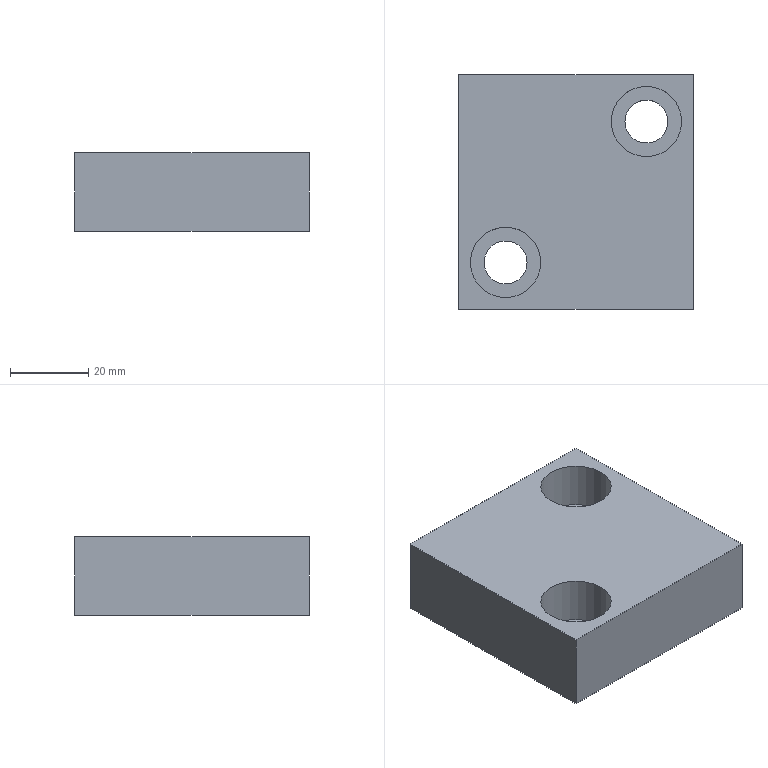Part | NX | features solid 2 | 1 solid | 12 faces | box 60 x 60 x 20 mm | volume 64372 mm3 | plane 8 | cylinder 4 | commonest cylinder face diameters 11 x2 18 x2
STEP:
#1=CARTESIAN_POINT('',(12.5,568.,142.));
#2=VERTEX_POINT('',#1);
#3=CARTESIAN_POINT('',(18.,568.,142.));
#4=DIRECTION('',(0.,0.,-1.));
#5=DIRECTION('',(-1.,0.,0.));
#6=AXIS2_PLACEMENT_3D('',#3,#4,#5);
#7=CIRCLE('',#6,5.5);
#8=EDGE_CURVE('',#2,#2,#7,.T.);
#9=ORIENTED_EDGE('',*,*,#8,.F.);
#10=EDGE_LOOP('',(#9));
#11=FACE_BOUND('',#10,.T.);
#12=CARTESIAN_POINT('',(-23.5,532.,142.));
#13=VERTEX_POINT('',#12);
#14=CARTESIAN_POINT('',(-18.,532.,142.));
#15=DIRECTION('',(0.,0.,-1.));
#16=DIRECTION('',(-1.,0.,0.));
#17=AXIS2_PLACEMENT_3D('',#14,#15,#16);
#18=CIRCLE('',#17,5.5);
#19=EDGE_CURVE('',#13,#13,#18,.T.);
#20=ORIENTED_EDGE('',*,*,#19,.F.);
#21=EDGE_LOOP('',(#20));
#22=FACE_BOUND('',#21,.T.);
#23=CARTESIAN_POINT('',(-30.,520.,142.));
#24=VERTEX_POINT('',#23);
#25=CARTESIAN_POINT('',(30.,520.,142.));
#26=VERTEX_POINT('',#25);
#27=CARTESIAN_POINT('',(-37.5,520.,142.));
#28=DIRECTION('',(-1.,0.,0.));
#29=VECTOR('',#28,1000.);
#30=LINE('',#27,#29);
#31=EDGE_CURVE('',#24,#26,#30,.F.);
#32=ORIENTED_EDGE('',*,*,#31,.F.);
#33=CARTESIAN_POINT('',(-30.,580.,142.));
#34=VERTEX_POINT('',#33);
#35=CARTESIAN_POINT('',(-30.,600.,142.));
#36=DIRECTION('',(0.,1.,0.));
#37=VECTOR('',#36,1000.);
#38=LINE('',#35,#37);
#39=EDGE_CURVE('',#34,#24,#38,.F.);
#40=ORIENTED_EDGE('',*,*,#39,.F.);
#41=CARTESIAN_POINT('',(30.,580.,142.));
#42=VERTEX_POINT('',#41);
#43=CARTESIAN_POINT('',(-37.5,580.,142.));
#44=DIRECTION('',(1.,0.,0.));
#45=VECTOR('',#44,1000.);
#46=LINE('',#43,#45);
#47=EDGE_CURVE('',#34,#42,#46,.T.);
#48=ORIENTED_EDGE('',*,*,#47,.T.);
#49=CARTESIAN_POINT('',(30.,600.,142.));
#50=DIRECTION('',(0.,-1.,0.));
#51=VECTOR('',#50,1000.);
#52=LINE('',#49,#51);
#53=EDGE_CURVE('',#42,#26,#52,.T.);
#54=ORIENTED_EDGE('',*,*,#53,.T.);
#55=EDGE_LOOP('',(#32,#40,#48,#54));
#56=FACE_BOUND('',#55,.T.);
#57=CARTESIAN_POINT('',(-37.5,600.,142.));
#58=DIRECTION('',(0.,0.,-1.));
#59=DIRECTION('',(-1.,0.,0.));
#60=AXIS2_PLACEMENT_3D('',#57,#58,#59);
#61=PLANE('',#60);
#62=ADVANCED_FACE('',(#11,#22,#56),#61,.T.);
#63=CARTESIAN_POINT('',(30.,580.,162.));
#64=VERTEX_POINT('',#63);
#65=CARTESIAN_POINT('',(30.,580.,142.));
#66=DIRECTION('',(0.,0.,1.));
#67=VECTOR('',#66,1000.);
#68=LINE('',#65,#67);
#69=EDGE_CURVE('',#42,#64,#68,.T.);
#70=ORIENTED_EDGE('',*,*,#69,.F.);
#71=ORIENTED_EDGE('',*,*,#47,.F.);
#72=CARTESIAN_POINT('',(-30.,580.,162.));
#73=VERTEX_POINT('',#72);
#74=CARTESIAN_POINT('',(-30.,580.,142.));
#75=DIRECTION('',(0.,0.,-1.));
#76=VECTOR('',#75,1000.);
#77=LINE('',#74,#76);
#78=EDGE_CURVE('',#34,#73,#77,.F.);
#79=ORIENTED_EDGE('',*,*,#78,.T.);
#80=CARTESIAN_POINT('',(-37.5,580.,162.));
#81=DIRECTION('',(1.,0.,0.));
#82=VECTOR('',#81,1000.);
#83=LINE('',#80,#82);
#84=EDGE_CURVE('',#73,#64,#83,.T.);
#85=ORIENTED_EDGE('',*,*,#84,.T.);
#86=EDGE_LOOP('',(#70,#71,#79,#85));
#87=FACE_BOUND('',#86,.T.);
#88=CARTESIAN_POINT('',(-37.5,580.,142.));
#89=DIRECTION('',(0.,1.,0.));
#90=DIRECTION('',(1.,0.,0.));
#91=AXIS2_PLACEMENT_3D('',#88,#89,#90);
#92=PLANE('',#91);
#93=ADVANCED_FACE('',(#87),#92,.T.);
#94=ORIENTED_EDGE('',*,*,#78,.F.);
#95=ORIENTED_EDGE('',*,*,#39,.T.);
#96=CARTESIAN_POINT('',(-30.,520.,162.));
#97=VERTEX_POINT('',#96);
#98=CARTESIAN_POINT('',(-30.,520.,142.));
#99=DIRECTION('',(0.,0.,1.));
#100=VECTOR('',#99,1000.);
#101=LINE('',#98,#100);
#102=EDGE_CURVE('',#24,#97,#101,.T.);
#103=ORIENTED_EDGE('',*,*,#102,.T.);
#104=CARTESIAN_POINT('',(-30.,600.,162.));
#105=DIRECTION('',(0.,1.,0.));
#106=VECTOR('',#105,1000.);
#107=LINE('',#104,#106);
#108=EDGE_CURVE('',#73,#97,#107,.F.);
#109=ORIENTED_EDGE('',*,*,#108,.F.);
#110=EDGE_LOOP('',(#94,#95,#103,#109));
#111=FACE_BOUND('',#110,.T.);
#112=CARTESIAN_POINT('',(-30.,600.,142.));
#113=DIRECTION('',(1.,0.,0.));
#114=DIRECTION('',(0.,-1.,0.));
#115=AXIS2_PLACEMENT_3D('',#112,#113,#114);
#116=PLANE('',#115);
#117=ADVANCED_FACE('',(#111),#116,.F.);
#118=ORIENTED_EDGE('',*,*,#102,.F.);
#119=ORIENTED_EDGE('',*,*,#31,.T.);
#120=CARTESIAN_POINT('',(30.,520.,162.));
#121=VERTEX_POINT('',#120);
#122=CARTESIAN_POINT('',(30.,520.,142.));
#123=DIRECTION('',(0.,0.,-1.));
#124=VECTOR('',#123,1000.);
#125=LINE('',#122,#124);
#126=EDGE_CURVE('',#26,#121,#125,.F.);
#127=ORIENTED_EDGE('',*,*,#126,.T.);
#128=CARTESIAN_POINT('',(-37.5,520.,162.));
#129=DIRECTION('',(-1.,0.,0.));
#130=VECTOR('',#129,1000.);
#131=LINE('',#128,#130);
#132=EDGE_CURVE('',#97,#121,#131,.F.);
#133=ORIENTED_EDGE('',*,*,#132,.F.);
#134=EDGE_LOOP('',(#118,#119,#127,#133));
#135=FACE_BOUND('',#134,.T.);
#136=CARTESIAN_POINT('',(-37.5,520.,142.));
#137=DIRECTION('',(0.,1.,0.));
#138=DIRECTION('',(1.,0.,0.));
#139=AXIS2_PLACEMENT_3D('',#136,#137,#138);
#140=PLANE('',#139);
#141=ADVANCED_FACE('',(#135),#140,.F.);
#142=CARTESIAN_POINT('',(9.,568.,162.));
#143=VERTEX_POINT('',#142);
#144=CARTESIAN_POINT('',(18.,568.,162.));
#145=DIRECTION('',(0.,0.,-1.));
#146=DIRECTION('',(-1.,0.,0.));
#147=AXIS2_PLACEMENT_3D('',#144,#145,#146);
#148=CIRCLE('',#147,9.);
#149=EDGE_CURVE('',#143,#143,#148,.T.);
#150=ORIENTED_EDGE('',*,*,#149,.T.);
#151=EDGE_LOOP('',(#150));
#152=FACE_BOUND('',#151,.T.);
#153=CARTESIAN_POINT('',(-27.,532.,162.));
#154=VERTEX_POINT('',#153);
#155=CARTESIAN_POINT('',(-18.,532.,162.));
#156=DIRECTION('',(0.,0.,-1.));
#157=DIRECTION('',(-1.,0.,0.));
#158=AXIS2_PLACEMENT_3D('',#155,#156,#157);
#159=CIRCLE('',#158,9.);
#160=EDGE_CURVE('',#154,#154,#159,.T.);
#161=ORIENTED_EDGE('',*,*,#160,.T.);
#162=EDGE_LOOP('',(#161));
#163=FACE_BOUND('',#162,.T.);
#164=ORIENTED_EDGE('',*,*,#132,.T.);
#165=CARTESIAN_POINT('',(30.,600.,162.));
#166=DIRECTION('',(0.,-1.,0.));
#167=VECTOR('',#166,1000.);
#168=LINE('',#165,#167);
#169=EDGE_CURVE('',#64,#121,#168,.T.);
#170=ORIENTED_EDGE('',*,*,#169,.F.);
#171=ORIENTED_EDGE('',*,*,#84,.F.);
#172=ORIENTED_EDGE('',*,*,#108,.T.);
#173=EDGE_LOOP('',(#164,#170,#171,#172));
#174=FACE_BOUND('',#173,.T.);
#175=CARTESIAN_POINT('',(-37.5,600.,162.));
#176=DIRECTION('',(0.,0.,-1.));
#177=DIRECTION('',(-1.,0.,0.));
#178=AXIS2_PLACEMENT_3D('',#175,#176,#177);
#179=PLANE('',#178);
#180=ADVANCED_FACE('',(#152,#163,#174),#179,.F.);
#181=ORIENTED_EDGE('',*,*,#53,.F.);
#182=ORIENTED_EDGE('',*,*,#69,.T.);
#183=ORIENTED_EDGE('',*,*,#169,.T.);
#184=ORIENTED_EDGE('',*,*,#126,.F.);
#185=EDGE_LOOP('',(#181,#182,#183,#184));
#186=FACE_BOUND('',#185,.T.);
#187=CARTESIAN_POINT('',(30.,600.,142.));
#188=DIRECTION('',(1.,0.,0.));
#189=DIRECTION('',(0.,-1.,0.));
#190=AXIS2_PLACEMENT_3D('',#187,#188,#189);
#191=PLANE('',#190);
#192=ADVANCED_FACE('',(#186),#191,.T.);
#193=ORIENTED_EDGE('',*,*,#19,.T.);
#194=EDGE_LOOP('',(#193));
#195=FACE_BOUND('',#194,.T.);
#196=CARTESIAN_POINT('',(-23.5,532.,150.));
#197=VERTEX_POINT('',#196);
#198=CARTESIAN_POINT('',(-18.,532.,150.));
#199=DIRECTION('',(0.,0.,-1.));
#200=DIRECTION('',(-1.,0.,0.));
#201=AXIS2_PLACEMENT_3D('',#198,#199,#200);
#202=CIRCLE('',#201,5.5);
#203=EDGE_CURVE('',#197,#197,#202,.T.);
#204=ORIENTED_EDGE('',*,*,#203,.F.);
#205=EDGE_LOOP('',(#204));
#206=FACE_BOUND('',#205,.T.);
#207=CARTESIAN_POINT('',(-18.,532.,62.));
#208=DIRECTION('',(0.,0.,-1.));
#209=DIRECTION('',(-1.,0.,0.));
#210=AXIS2_PLACEMENT_3D('',#207,#208,#209);
#211=CYLINDRICAL_SURFACE('',#210,5.5);
#212=ADVANCED_FACE('',(#195,#206),#211,.F.);
#213=ORIENTED_EDGE('',*,*,#203,.T.);
#214=EDGE_LOOP('',(#213));
#215=FACE_BOUND('',#214,.T.);
#216=CARTESIAN_POINT('',(-27.,532.,150.));
#217=VERTEX_POINT('',#216);
#218=CARTESIAN_POINT('',(-18.,532.,150.));
#219=DIRECTION('',(0.,0.,-1.));
#220=DIRECTION('',(-1.,0.,0.));
#221=AXIS2_PLACEMENT_3D('',#218,#219,#220);
#222=CIRCLE('',#221,9.);
#223=EDGE_CURVE('',#217,#217,#222,.T.);
#224=ORIENTED_EDGE('',*,*,#223,.F.);
#225=EDGE_LOOP('',(#224));
#226=FACE_BOUND('',#225,.T.);
#227=CARTESIAN_POINT('',(18.,568.,150.));
#228=DIRECTION('',(0.,0.,-1.));
#229=DIRECTION('',(-1.,0.,0.));
#230=AXIS2_PLACEMENT_3D('',#227,#228,#229);
#231=PLANE('',#230);
#232=ADVANCED_FACE('',(#215,#226),#231,.F.);
#233=ORIENTED_EDGE('',*,*,#223,.T.);
#234=EDGE_LOOP('',(#233));
#235=FACE_BOUND('',#234,.T.);
#236=ORIENTED_EDGE('',*,*,#160,.F.);
#237=EDGE_LOOP('',(#236));
#238=FACE_BOUND('',#237,.T.);
#239=CARTESIAN_POINT('',(-18.,532.,162.));
#240=DIRECTION('',(0.,0.,-1.));
#241=DIRECTION('',(-1.,0.,0.));
#242=AXIS2_PLACEMENT_3D('',#239,#240,#241);
#243=CYLINDRICAL_SURFACE('',#242,9.);
#244=ADVANCED_FACE('',(#235,#238),#243,.F.);
#245=ORIENTED_EDGE('',*,*,#8,.T.);
#246=EDGE_LOOP('',(#245));
#247=FACE_BOUND('',#246,.T.);
#248=CARTESIAN_POINT('',(12.5,568.,150.));
#249=VERTEX_POINT('',#248);
#250=CARTESIAN_POINT('',(18.,568.,150.));
#251=DIRECTION('',(0.,0.,-1.));
#252=DIRECTION('',(-1.,0.,0.));
#253=AXIS2_PLACEMENT_3D('',#250,#251,#252);
#254=CIRCLE('',#253,5.5);
#255=EDGE_CURVE('',#249,#249,#254,.T.);
#256=ORIENTED_EDGE('',*,*,#255,.F.);
#257=EDGE_LOOP('',(#256));
#258=FACE_BOUND('',#257,.T.);
#259=CARTESIAN_POINT('',(18.,568.,62.));
#260=DIRECTION('',(0.,0.,-1.));
#261=DIRECTION('',(-1.,0.,0.));
#262=AXIS2_PLACEMENT_3D('',#259,#260,#261);
#263=CYLINDRICAL_SURFACE('',#262,5.5);
#264=ADVANCED_FACE('',(#247,#258),#263,.F.);
#265=ORIENTED_EDGE('',*,*,#255,.T.);
#266=EDGE_LOOP('',(#265));
#267=FACE_BOUND('',#266,.T.);
#268=CARTESIAN_POINT('',(9.,568.,150.));
#269=VERTEX_POINT('',#268);
#270=CARTESIAN_POINT('',(18.,568.,150.));
#271=DIRECTION('',(0.,0.,-1.));
#272=DIRECTION('',(-1.,0.,0.));
#273=AXIS2_PLACEMENT_3D('',#270,#271,#272);
#274=CIRCLE('',#273,9.);
#275=EDGE_CURVE('',#269,#269,#274,.T.);
#276=ORIENTED_EDGE('',*,*,#275,.F.);
#277=EDGE_LOOP('',(#276));
#278=FACE_BOUND('',#277,.T.);
#279=CARTESIAN_POINT('',(18.,568.,150.));
#280=DIRECTION('',(0.,0.,-1.));
#281=DIRECTION('',(-1.,0.,0.));
#282=AXIS2_PLACEMENT_3D('',#279,#280,#281);
#283=PLANE('',#282);
#284=ADVANCED_FACE('',(#267,#278),#283,.F.);
#285=ORIENTED_EDGE('',*,*,#275,.T.);
#286=EDGE_LOOP('',(#285));
#287=FACE_BOUND('',#286,.T.);
#288=ORIENTED_EDGE('',*,*,#149,.F.);
#289=EDGE_LOOP('',(#288));
#290=FACE_BOUND('',#289,.T.);
#291=CARTESIAN_POINT('',(18.,568.,162.));
#292=DIRECTION('',(0.,0.,-1.));
#293=DIRECTION('',(-1.,0.,0.));
#294=AXIS2_PLACEMENT_3D('',#291,#292,#293);
#295=CYLINDRICAL_SURFACE('',#294,9.);
#296=ADVANCED_FACE('',(#287,#290),#295,.F.);
#297=CLOSED_SHELL('',(#62,#93,#117,#141,#180,#192,#212,#232,#244,#264,#284,#296));
#298=MANIFOLD_SOLID_BREP('',#297);
#299=(LENGTH_UNIT()NAMED_UNIT(*)SI_UNIT(.MILLI.,.METRE.));
#300=UNCERTAINTY_MEASURE_WITH_UNIT(LENGTH_MEASURE(0.00001),#299,'','');
#301=(NAMED_UNIT(*)PLANE_ANGLE_UNIT()SI_UNIT($,.RADIAN.));
#302=(NAMED_UNIT(*)SI_UNIT($,.STERADIAN.)SOLID_ANGLE_UNIT());
#303=(GEOMETRIC_REPRESENTATION_CONTEXT(3)GLOBAL_UNCERTAINTY_ASSIGNED_CONTEXT((#300))GLOBAL_UNIT_ASSIGNED_CONTEXT((#299,#301,#302))REPRESENTATION_CONTEXT('',''));
#304=ADVANCED_BREP_SHAPE_REPRESENTATION('',(#298),#303);